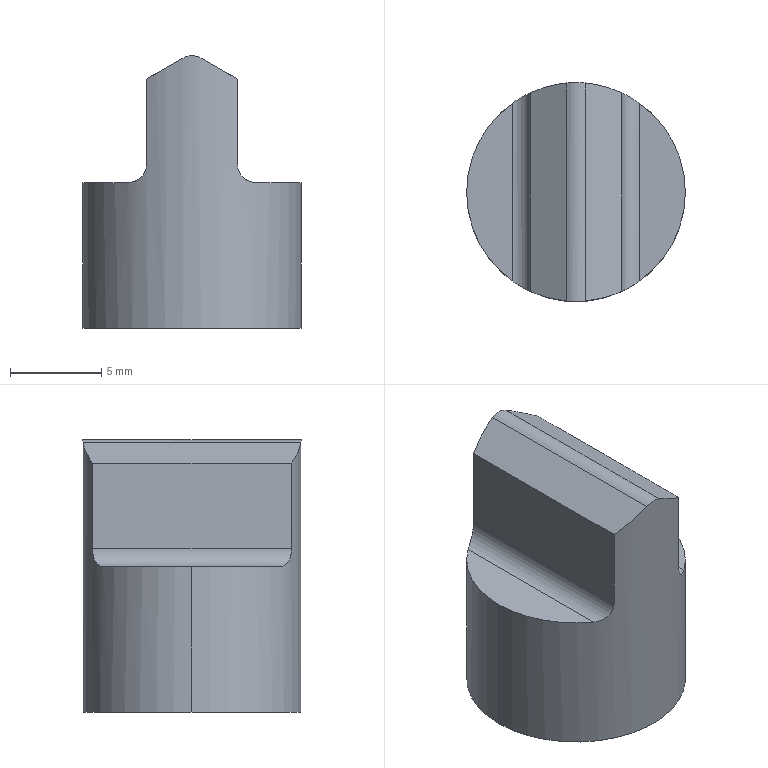Part | Creo | 1 solid | 15 faces | box 12 x 12 x 14.965 mm | volume 1022 mm3 | plane 8 | cylinder 7 | commonest cylinder face diameters 2 x3 10.5 x2 12 x2
STEP:
#1=CARTESIAN_POINT('',(257.5,-185.454,-31.823));
#2=VERTEX_POINT('',#1);
#3=CARTESIAN_POINT('',(257.5,-185.454,-36.5));
#4=VERTEX_POINT('',#3);
#5=CARTESIAN_POINT('',(257.5,-185.454,-31.823));
#6=DIRECTION('',(0.,0.,-1.));
#7=VECTOR('',#6,4.677);
#8=LINE('',#5,#7);
#9=EDGE_CURVE('',#2,#4,#8,.T.);
#10=ORIENTED_EDGE('',*,*,#9,.T.);
#11=CARTESIAN_POINT('',(257.5,-174.546,-36.5));
#12=VERTEX_POINT('',#11);
#13=CARTESIAN_POINT('',(257.5,-185.454,-36.5));
#14=DIRECTION('',(0.,1.,0.));
#15=VECTOR('',#14,10.909);
#16=LINE('',#13,#15);
#17=EDGE_CURVE('',#4,#12,#16,.T.);
#18=ORIENTED_EDGE('',*,*,#17,.T.);
#19=CARTESIAN_POINT('',(257.5,-174.546,-31.823));
#20=VERTEX_POINT('',#19);
#21=CARTESIAN_POINT('',(257.5,-174.546,-36.5));
#22=DIRECTION('',(0.,0.,1.));
#23=VECTOR('',#22,4.677);
#24=LINE('',#21,#23);
#25=EDGE_CURVE('',#12,#20,#24,.T.);
#26=ORIENTED_EDGE('',*,*,#25,.T.);
#27=CARTESIAN_POINT('',(257.5,-174.546,-31.823));
#28=DIRECTION('',(0.,-1.,0.));
#29=VECTOR('',#28,10.909);
#30=LINE('',#27,#29);
#31=EDGE_CURVE('',#20,#2,#30,.T.);
#32=ORIENTED_EDGE('',*,*,#31,.T.);
#33=EDGE_LOOP('',(#10,#18,#26,#32));
#34=FACE_OUTER_BOUND('',#33,.F.);
#35=CARTESIAN_POINT('',(257.5,-180.,-45.5));
#36=DIRECTION('',(1.,0.,0.));
#37=DIRECTION('',(0.,0.,-1.));
#38=AXIS2_PLACEMENT_3D('',#35,#36,#37);
#39=PLANE('',#38);
#40=ADVANCED_FACE('',(#34),#39,.F.);
#41=CARTESIAN_POINT('',(263.5,-184.873,-37.5));
#42=VERTEX_POINT('',#41);
#43=CARTESIAN_POINT('',(266.,-180.,-37.5));
#44=VERTEX_POINT('',#43);
#45=CARTESIAN_POINT('',(260.,-180.,-37.5));
#46=DIRECTION('',(0.,0.,1.));
#47=DIRECTION('',(0.5833,-0.8122,0.));
#48=AXIS2_PLACEMENT_3D('',#45,#46,#47);
#49=CIRCLE('',#48,6.);
#50=EDGE_CURVE('',#42,#44,#49,.T.);
#51=ORIENTED_EDGE('',*,*,#50,.T.);
#52=CARTESIAN_POINT('',(266.,-180.,-45.5));
#53=VERTEX_POINT('',#52);
#54=CARTESIAN_POINT('',(266.,-180.,-45.5));
#55=DIRECTION('',(0.,0.,1.));
#56=VECTOR('',#55,8.);
#57=LINE('',#54,#56);
#58=EDGE_CURVE('',#53,#44,#57,.T.);
#59=ORIENTED_EDGE('',*,*,#58,.F.);
#60=CARTESIAN_POINT('',(254.,-180.,-45.5));
#61=VERTEX_POINT('',#60);
#62=CARTESIAN_POINT('',(260.,-180.,-45.5));
#63=DIRECTION('',(0.,0.,-1.));
#64=DIRECTION('',(1.,0.,0.));
#65=AXIS2_PLACEMENT_3D('',#62,#63,#64);
#66=CIRCLE('',#65,6.);
#67=EDGE_CURVE('',#53,#61,#66,.T.);
#68=ORIENTED_EDGE('',*,*,#67,.T.);
#69=CARTESIAN_POINT('',(254.,-180.,-37.5));
#70=VERTEX_POINT('',#69);
#71=CARTESIAN_POINT('',(254.,-180.,-45.5));
#72=DIRECTION('',(0.000002775,0.,1.));
#73=VECTOR('',#72,8.);
#74=LINE('',#71,#73);
#75=EDGE_CURVE('',#61,#70,#74,.T.);
#76=ORIENTED_EDGE('',*,*,#75,.T.);
#77=CARTESIAN_POINT('',(256.5,-184.873,-37.5));
#78=VERTEX_POINT('',#77);
#79=CARTESIAN_POINT('',(260.,-180.,-37.5));
#80=DIRECTION('',(0.,0.,1.));
#81=DIRECTION('',(-1.,0.,0.));
#82=AXIS2_PLACEMENT_3D('',#79,#80,#81);
#83=CIRCLE('',#82,6.);
#84=EDGE_CURVE('',#70,#78,#83,.T.);
#85=ORIENTED_EDGE('',*,*,#84,.T.);
#86=CARTESIAN_POINT('',(257.5,-185.454,-36.5));
#87=CARTESIAN_POINT('',(257.5,-185.454,-36.573));
#88=CARTESIAN_POINT('',(257.484,-185.447,-36.716));
#89=CARTESIAN_POINT('',(257.414,-185.414,-36.926));
#90=CARTESIAN_POINT('',(257.299,-185.358,-37.115));
#91=CARTESIAN_POINT('',(257.144,-185.278,-37.276));
#92=CARTESIAN_POINT('',(256.954,-185.171,-37.401));
#93=CARTESIAN_POINT('',(256.737,-185.038,-37.481));
#94=CARTESIAN_POINT('',(256.581,-184.932,-37.5));
#95=CARTESIAN_POINT('',(256.5,-184.873,-37.5));
#96=B_SPLINE_CURVE_WITH_KNOTS('',3,(#86,#87,#88,#89,#90,#91,#92,#93,#94,#95),.UNSPECIFIED.,.F.,.F.,(4,1,1,1,1,1,1,4),(0.,0.1429,0.2857,0.4286,0.5714,0.7143,0.8571,1.),.UNSPECIFIED.);
#97=EDGE_CURVE('',#4,#78,#96,.T.);
#98=ORIENTED_EDGE('',*,*,#97,.F.);
#99=ORIENTED_EDGE('',*,*,#9,.F.);
#100=CARTESIAN_POINT('',(259.5,-185.979,-30.669));
#101=VERTEX_POINT('',#100);
#102=CARTESIAN_POINT('',(259.5,-185.979,-30.669));
#103=CARTESIAN_POINT('',(258.81,-185.921,-31.067));
#104=CARTESIAN_POINT('',(258.143,-185.749,-31.452));
#105=CARTESIAN_POINT('',(257.5,-185.454,-31.823));
#106=B_SPLINE_CURVE_WITH_KNOTS('',3,(#102,#103,#104,#105),.UNSPECIFIED.,.F.,.F.,(4,4),(0.,1.),.UNSPECIFIED.);
#107=EDGE_CURVE('',#101,#2,#106,.T.);
#108=ORIENTED_EDGE('',*,*,#107,.F.);
#109=CARTESIAN_POINT('',(260.5,-185.979,-30.669));
#110=VERTEX_POINT('',#109);
#111=CARTESIAN_POINT('',(260.5,-185.979,-30.669));
#112=CARTESIAN_POINT('',(260.439,-185.984,-30.633));
#113=CARTESIAN_POINT('',(260.311,-185.993,-30.577));
#114=CARTESIAN_POINT('',(260.105,-186.,-30.533));
#115=CARTESIAN_POINT('',(259.896,-186.,-30.533));
#116=CARTESIAN_POINT('',(259.689,-185.993,-30.577));
#117=CARTESIAN_POINT('',(259.562,-185.984,-30.633));
#118=CARTESIAN_POINT('',(259.5,-185.979,-30.669));
#119=B_SPLINE_CURVE_WITH_KNOTS('',3,(#111,#112,#113,#114,#115,#116,#117,#118),.UNSPECIFIED.,.F.,.F.,(4,1,1,1,1,4),(0.,0.2,0.4,0.6,0.8,1.),.UNSPECIFIED.);
#120=EDGE_CURVE('',#110,#101,#119,.T.);
#121=ORIENTED_EDGE('',*,*,#120,.F.);
#122=CARTESIAN_POINT('',(262.5,-185.454,-31.823));
#123=VERTEX_POINT('',#122);
#124=CARTESIAN_POINT('',(260.5,-185.979,-30.669));
#125=CARTESIAN_POINT('',(261.19,-185.921,-31.067));
#126=CARTESIAN_POINT('',(261.857,-185.749,-31.452));
#127=CARTESIAN_POINT('',(262.5,-185.454,-31.823));
#128=B_SPLINE_CURVE_WITH_KNOTS('',3,(#124,#125,#126,#127),.UNSPECIFIED.,.F.,.F.,(4,4),(0.,1.),.UNSPECIFIED.);
#129=EDGE_CURVE('',#110,#123,#128,.T.);
#130=ORIENTED_EDGE('',*,*,#129,.T.);
#131=CARTESIAN_POINT('',(262.5,-185.454,-36.5));
#132=VERTEX_POINT('',#131);
#133=CARTESIAN_POINT('',(262.5,-185.454,-36.5));
#134=DIRECTION('',(0.,0.,1.));
#135=VECTOR('',#134,4.677);
#136=LINE('',#133,#135);
#137=EDGE_CURVE('',#132,#123,#136,.T.);
#138=ORIENTED_EDGE('',*,*,#137,.F.);
#139=CARTESIAN_POINT('',(263.5,-184.873,-37.5));
#140=CARTESIAN_POINT('',(263.419,-184.932,-37.5));
#141=CARTESIAN_POINT('',(263.262,-185.038,-37.48));
#142=CARTESIAN_POINT('',(263.045,-185.172,-37.4));
#143=CARTESIAN_POINT('',(262.855,-185.278,-37.275));
#144=CARTESIAN_POINT('',(262.7,-185.359,-37.114));
#145=CARTESIAN_POINT('',(262.586,-185.414,-36.925));
#146=CARTESIAN_POINT('',(262.516,-185.447,-36.717));
#147=CARTESIAN_POINT('',(262.5,-185.454,-36.573));
#148=CARTESIAN_POINT('',(262.5,-185.454,-36.5));
#149=B_SPLINE_CURVE_WITH_KNOTS('',3,(#139,#140,#141,#142,#143,#144,#145,#146,#147,#148),.UNSPECIFIED.,.F.,.F.,(4,1,1,1,1,1,1,4),(0.,0.1429,0.2857,0.4286,0.5714,0.7143,0.8571,1.),.UNSPECIFIED.);
#150=EDGE_CURVE('',#42,#132,#149,.T.);
#151=ORIENTED_EDGE('',*,*,#150,.F.);
#152=EDGE_LOOP('',(#51,#59,#68,#76,#85,#98,#99,#108,#121,#130,#138,#151));
#153=FACE_OUTER_BOUND('',#152,.F.);
#154=CARTESIAN_POINT('',(260.,-180.,-53.5));
#155=DIRECTION('',(0.,0.,1.));
#156=DIRECTION('',(1.,0.,0.));
#157=AXIS2_PLACEMENT_3D('',#154,#155,#156);
#158=CYLINDRICAL_SURFACE('',#157,6.);
#159=ADVANCED_FACE('',(#153),#158,.T.);
#160=ORIENTED_EDGE('',*,*,#50,.F.);
#161=CARTESIAN_POINT('',(263.5,-175.127,-37.5));
#162=VERTEX_POINT('',#161);
#163=CARTESIAN_POINT('',(263.5,-184.873,-37.5));
#164=DIRECTION('',(0.,1.,0.));
#165=VECTOR('',#164,9.747);
#166=LINE('',#163,#165);
#167=EDGE_CURVE('',#42,#162,#166,.T.);
#168=ORIENTED_EDGE('',*,*,#167,.T.);
#169=CARTESIAN_POINT('',(260.,-180.,-37.5));
#170=DIRECTION('',(0.,0.,1.));
#171=DIRECTION('',(1.,0.,0.));
#172=AXIS2_PLACEMENT_3D('',#169,#170,#171);
#173=CIRCLE('',#172,6.);
#174=EDGE_CURVE('',#44,#162,#173,.T.);
#175=ORIENTED_EDGE('',*,*,#174,.F.);
#176=EDGE_LOOP('',(#160,#168,#175));
#177=FACE_OUTER_BOUND('',#176,.F.);
#178=CARTESIAN_POINT('',(260.,-180.,-37.5));
#179=DIRECTION('',(0.,0.,1.));
#180=DIRECTION('',(-1.,0.,0.));
#181=AXIS2_PLACEMENT_3D('',#178,#179,#180);
#182=PLANE('',#181);
#183=ADVANCED_FACE('',(#177),#182,.T.);
#184=CARTESIAN_POINT('',(262.5,-174.546,-36.5));
#185=VERTEX_POINT('',#184);
#186=CARTESIAN_POINT('',(262.5,-174.546,-36.5));
#187=CARTESIAN_POINT('',(262.5,-174.546,-36.573));
#188=CARTESIAN_POINT('',(262.516,-174.553,-36.716));
#189=CARTESIAN_POINT('',(262.586,-174.586,-36.926));
#190=CARTESIAN_POINT('',(262.701,-174.642,-37.115));
#191=CARTESIAN_POINT('',(262.856,-174.722,-37.276));
#192=CARTESIAN_POINT('',(263.046,-174.829,-37.401));
#193=CARTESIAN_POINT('',(263.263,-174.962,-37.481));
#194=CARTESIAN_POINT('',(263.419,-175.068,-37.5));
#195=CARTESIAN_POINT('',(263.5,-175.127,-37.5));
#196=B_SPLINE_CURVE_WITH_KNOTS('',3,(#186,#187,#188,#189,#190,#191,#192,#193,#194,#195),.UNSPECIFIED.,.F.,.F.,(4,1,1,1,1,1,1,4),(0.,0.1429,0.2857,0.4286,0.5714,0.7143,0.8571,1.),.UNSPECIFIED.);
#197=EDGE_CURVE('',#185,#162,#196,.T.);
#198=ORIENTED_EDGE('',*,*,#197,.T.);
#199=ORIENTED_EDGE('',*,*,#167,.F.);
#200=ORIENTED_EDGE('',*,*,#150,.T.);
#201=CARTESIAN_POINT('',(262.5,-174.546,-36.5));
#202=DIRECTION('',(0.,-1.,0.));
#203=VECTOR('',#202,10.909);
#204=LINE('',#201,#203);
#205=EDGE_CURVE('',#185,#132,#204,.T.);
#206=ORIENTED_EDGE('',*,*,#205,.F.);
#207=EDGE_LOOP('',(#198,#199,#200,#206));
#208=FACE_OUTER_BOUND('',#207,.F.);
#209=CARTESIAN_POINT('',(263.5,-180.,-36.5));
#210=DIRECTION('',(0.,-1.,0.));
#211=DIRECTION('',(0.,0.,-1.));
#212=AXIS2_PLACEMENT_3D('',#209,#210,#211);
#213=CYLINDRICAL_SURFACE('',#212,1.);
#214=ADVANCED_FACE('',(#208),#213,.F.);
#215=CARTESIAN_POINT('',(262.5,-174.546,-31.823));
#216=VERTEX_POINT('',#215);
#217=CARTESIAN_POINT('',(260.5,-174.021,-30.669));
#218=VERTEX_POINT('',#217);
#219=CARTESIAN_POINT('',(262.5,-174.546,-31.823));
#220=CARTESIAN_POINT('',(261.857,-174.251,-31.452));
#221=CARTESIAN_POINT('',(261.19,-174.079,-31.067));
#222=CARTESIAN_POINT('',(260.5,-174.021,-30.669));
#223=B_SPLINE_CURVE_WITH_KNOTS('',3,(#219,#220,#221,#222),.UNSPECIFIED.,.F.,.F.,(4,4),(0.,1.),.UNSPECIFIED.);
#224=EDGE_CURVE('',#216,#218,#223,.T.);
#225=ORIENTED_EDGE('',*,*,#224,.T.);
#226=CARTESIAN_POINT('',(259.5,-174.021,-30.669));
#227=VERTEX_POINT('',#226);
#228=CARTESIAN_POINT('',(259.5,-174.021,-30.669));
#229=CARTESIAN_POINT('',(259.561,-174.016,-30.633));
#230=CARTESIAN_POINT('',(259.689,-174.007,-30.577));
#231=CARTESIAN_POINT('',(259.895,-174.,-30.533));
#232=CARTESIAN_POINT('',(260.104,-174.,-30.533));
#233=CARTESIAN_POINT('',(260.311,-174.007,-30.577));
#234=CARTESIAN_POINT('',(260.438,-174.016,-30.633));
#235=CARTESIAN_POINT('',(260.5,-174.021,-30.669));
#236=B_SPLINE_CURVE_WITH_KNOTS('',3,(#228,#229,#230,#231,#232,#233,#234,#235),.UNSPECIFIED.,.F.,.F.,(4,1,1,1,1,4),(0.,0.2,0.4,0.6,0.8,1.),.UNSPECIFIED.);
#237=EDGE_CURVE('',#227,#218,#236,.T.);
#238=ORIENTED_EDGE('',*,*,#237,.F.);
#239=CARTESIAN_POINT('',(257.5,-174.546,-31.823));
#240=CARTESIAN_POINT('',(258.143,-174.251,-31.452));
#241=CARTESIAN_POINT('',(258.81,-174.079,-31.067));
#242=CARTESIAN_POINT('',(259.5,-174.021,-30.669));
#243=B_SPLINE_CURVE_WITH_KNOTS('',3,(#239,#240,#241,#242),.UNSPECIFIED.,.F.,.F.,(4,4),(0.,1.),.UNSPECIFIED.);
#244=EDGE_CURVE('',#20,#227,#243,.T.);
#245=ORIENTED_EDGE('',*,*,#244,.F.);
#246=ORIENTED_EDGE('',*,*,#25,.F.);
#247=CARTESIAN_POINT('',(256.5,-175.127,-37.5));
#248=VERTEX_POINT('',#247);
#249=CARTESIAN_POINT('',(256.5,-175.127,-37.5));
#250=CARTESIAN_POINT('',(256.581,-175.068,-37.5));
#251=CARTESIAN_POINT('',(256.738,-174.962,-37.48));
#252=CARTESIAN_POINT('',(256.955,-174.828,-37.4));
#253=CARTESIAN_POINT('',(257.145,-174.722,-37.275));
#254=CARTESIAN_POINT('',(257.3,-174.641,-37.114));
#255=CARTESIAN_POINT('',(257.414,-174.586,-36.925));
#256=CARTESIAN_POINT('',(257.484,-174.553,-36.717));
#257=CARTESIAN_POINT('',(257.5,-174.546,-36.573));
#258=CARTESIAN_POINT('',(257.5,-174.546,-36.5));
#259=B_SPLINE_CURVE_WITH_KNOTS('',3,(#249,#250,#251,#252,#253,#254,#255,#256,#257,#258),.UNSPECIFIED.,.F.,.F.,(4,1,1,1,1,1,1,4),(0.,0.1429,0.2857,0.4286,0.5714,0.7143,0.8571,1.),.UNSPECIFIED.);
#260=EDGE_CURVE('',#248,#12,#259,.T.);
#261=ORIENTED_EDGE('',*,*,#260,.F.);
#262=CARTESIAN_POINT('',(260.,-180.,-37.5));
#263=DIRECTION('',(0.,0.,1.));
#264=DIRECTION('',(-0.5833,0.8122,0.));
#265=AXIS2_PLACEMENT_3D('',#262,#263,#264);
#266=CIRCLE('',#265,6.);
#267=EDGE_CURVE('',#248,#70,#266,.T.);
#268=ORIENTED_EDGE('',*,*,#267,.T.);
#269=ORIENTED_EDGE('',*,*,#75,.F.);
#270=CARTESIAN_POINT('',(260.,-180.,-45.5));
#271=DIRECTION('',(0.,0.,-1.));
#272=DIRECTION('',(-1.,0.,0.));
#273=AXIS2_PLACEMENT_3D('',#270,#271,#272);
#274=CIRCLE('',#273,6.);
#275=EDGE_CURVE('',#61,#53,#274,.T.);
#276=ORIENTED_EDGE('',*,*,#275,.T.);
#277=ORIENTED_EDGE('',*,*,#58,.T.);
#278=ORIENTED_EDGE('',*,*,#174,.T.);
#279=ORIENTED_EDGE('',*,*,#197,.F.);
#280=CARTESIAN_POINT('',(262.5,-174.546,-31.823));
#281=DIRECTION('',(0.,0.,-1.));
#282=VECTOR('',#281,4.677);
#283=LINE('',#280,#282);
#284=EDGE_CURVE('',#216,#185,#283,.T.);
#285=ORIENTED_EDGE('',*,*,#284,.F.);
#286=EDGE_LOOP('',(#225,#238,#245,#246,#261,#268,#269,#276,#277,#278,#279,#285));
#287=FACE_OUTER_BOUND('',#286,.F.);
#288=CARTESIAN_POINT('',(260.,-180.,-53.5));
#289=DIRECTION('',(0.,0.,1.));
#290=DIRECTION('',(1.,0.,0.));
#291=AXIS2_PLACEMENT_3D('',#288,#289,#290);
#292=CYLINDRICAL_SURFACE('',#291,6.);
#293=ADVANCED_FACE('',(#287),#292,.T.);
#294=ORIENTED_EDGE('',*,*,#129,.F.);
#295=CARTESIAN_POINT('',(260.5,-185.979,-30.669));
#296=DIRECTION('',(0.,1.,0.));
#297=VECTOR('',#296,11.958);
#298=LINE('',#295,#297);
#299=EDGE_CURVE('',#110,#218,#298,.T.);
#300=ORIENTED_EDGE('',*,*,#299,.T.);
#301=ORIENTED_EDGE('',*,*,#224,.F.);
#302=CARTESIAN_POINT('',(262.5,-174.546,-31.823));
#303=DIRECTION('',(0.,-1.,0.));
#304=VECTOR('',#303,10.909);
#305=LINE('',#302,#304);
#306=EDGE_CURVE('',#216,#123,#305,.T.);
#307=ORIENTED_EDGE('',*,*,#306,.T.);
#308=EDGE_LOOP('',(#294,#300,#301,#307));
#309=FACE_OUTER_BOUND('',#308,.F.);
#310=CARTESIAN_POINT('',(260.,-180.,-30.38));
#311=DIRECTION('',(0.5,0.,0.866));
#312=DIRECTION('',(-0.866,0.,0.5));
#313=AXIS2_PLACEMENT_3D('',#310,#311,#312);
#314=PLANE('',#313);
#315=ADVANCED_FACE('',(#309),#314,.T.);
#316=ORIENTED_EDGE('',*,*,#120,.T.);
#317=CARTESIAN_POINT('',(259.5,-174.021,-30.669));
#318=DIRECTION('',(0.,-1.,0.));
#319=VECTOR('',#318,11.958);
#320=LINE('',#317,#319);
#321=EDGE_CURVE('',#227,#101,#320,.T.);
#322=ORIENTED_EDGE('',*,*,#321,.F.);
#323=ORIENTED_EDGE('',*,*,#237,.T.);
#324=ORIENTED_EDGE('',*,*,#299,.F.);
#325=EDGE_LOOP('',(#316,#322,#323,#324));
#326=FACE_OUTER_BOUND('',#325,.F.);
#327=CARTESIAN_POINT('',(260.,-180.,-31.535));
#328=DIRECTION('',(0.,1.,0.));
#329=DIRECTION('',(0.,0.,1.));
#330=AXIS2_PLACEMENT_3D('',#327,#328,#329);
#331=CYLINDRICAL_SURFACE('',#330,1.);
#332=ADVANCED_FACE('',(#326),#331,.T.);
#333=ORIENTED_EDGE('',*,*,#244,.T.);
#334=ORIENTED_EDGE('',*,*,#321,.T.);
#335=ORIENTED_EDGE('',*,*,#107,.T.);
#336=ORIENTED_EDGE('',*,*,#31,.F.);
#337=EDGE_LOOP('',(#333,#334,#335,#336));
#338=FACE_OUTER_BOUND('',#337,.F.);
#339=CARTESIAN_POINT('',(260.,-180.,-30.38));
#340=DIRECTION('',(-0.5,0.,0.866));
#341=DIRECTION('',(0.866,0.,0.5));
#342=AXIS2_PLACEMENT_3D('',#339,#340,#341);
#343=PLANE('',#342);
#344=ADVANCED_FACE('',(#338),#343,.T.);
#345=ORIENTED_EDGE('',*,*,#284,.T.);
#346=ORIENTED_EDGE('',*,*,#205,.T.);
#347=ORIENTED_EDGE('',*,*,#137,.T.);
#348=ORIENTED_EDGE('',*,*,#306,.F.);
#349=EDGE_LOOP('',(#345,#346,#347,#348));
#350=FACE_OUTER_BOUND('',#349,.F.);
#351=CARTESIAN_POINT('',(262.5,-180.,-45.5));
#352=DIRECTION('',(-1.,0.,0.));
#353=DIRECTION('',(0.,0.,-1.));
#354=AXIS2_PLACEMENT_3D('',#351,#352,#353);
#355=PLANE('',#354);
#356=ADVANCED_FACE('',(#350),#355,.F.);
#357=ORIENTED_EDGE('',*,*,#260,.T.);
#358=ORIENTED_EDGE('',*,*,#17,.F.);
#359=ORIENTED_EDGE('',*,*,#97,.T.);
#360=CARTESIAN_POINT('',(256.5,-175.127,-37.5));
#361=DIRECTION('',(0.,-1.,0.));
#362=VECTOR('',#361,9.747);
#363=LINE('',#360,#362);
#364=EDGE_CURVE('',#248,#78,#363,.T.);
#365=ORIENTED_EDGE('',*,*,#364,.F.);
#366=EDGE_LOOP('',(#357,#358,#359,#365));
#367=FACE_OUTER_BOUND('',#366,.F.);
#368=CARTESIAN_POINT('',(256.5,-180.,-36.5));
#369=DIRECTION('',(0.,-1.,0.));
#370=DIRECTION('',(0.,0.,-1.));
#371=AXIS2_PLACEMENT_3D('',#368,#369,#370);
#372=CYLINDRICAL_SURFACE('',#371,1.);
#373=ADVANCED_FACE('',(#367),#372,.F.);
#374=ORIENTED_EDGE('',*,*,#84,.F.);
#375=ORIENTED_EDGE('',*,*,#267,.F.);
#376=ORIENTED_EDGE('',*,*,#364,.T.);
#377=EDGE_LOOP('',(#374,#375,#376));
#378=FACE_OUTER_BOUND('',#377,.F.);
#379=CARTESIAN_POINT('',(260.,-180.,-37.5));
#380=DIRECTION('',(0.,0.,1.));
#381=DIRECTION('',(-1.,0.,0.));
#382=AXIS2_PLACEMENT_3D('',#379,#380,#381);
#383=PLANE('',#382);
#384=ADVANCED_FACE('',(#378),#383,.T.);
#385=ORIENTED_EDGE('',*,*,#275,.F.);
#386=ORIENTED_EDGE('',*,*,#67,.F.);
#387=EDGE_LOOP('',(#385,#386));
#388=FACE_OUTER_BOUND('',#387,.F.);
#389=CARTESIAN_POINT('',(254.75,-180.,-45.5));
#390=VERTEX_POINT('',#389);
#391=CARTESIAN_POINT('',(265.25,-180.,-45.5));
#392=VERTEX_POINT('',#391);
#393=CARTESIAN_POINT('',(260.,-180.,-45.5));
#394=DIRECTION('',(0.,0.,1.));
#395=DIRECTION('',(-1.,0.,0.));
#396=AXIS2_PLACEMENT_3D('',#393,#394,#395);
#397=CIRCLE('',#396,5.25);
#398=EDGE_CURVE('',#390,#392,#397,.T.);
#399=ORIENTED_EDGE('',*,*,#398,.F.);
#400=CARTESIAN_POINT('',(260.,-180.,-45.5));
#401=DIRECTION('',(0.,0.,1.));
#402=DIRECTION('',(1.,0.,0.));
#403=AXIS2_PLACEMENT_3D('',#400,#401,#402);
#404=CIRCLE('',#403,5.25);
#405=EDGE_CURVE('',#392,#390,#404,.T.);
#406=ORIENTED_EDGE('',*,*,#405,.F.);
#407=EDGE_LOOP('',(#399,#406));
#408=FACE_BOUND('',#407,.F.);
#409=CARTESIAN_POINT('',(260.,-180.,-45.5));
#410=DIRECTION('',(0.,0.,1.));
#411=DIRECTION('',(-1.,0.,0.));
#412=AXIS2_PLACEMENT_3D('',#409,#410,#411);
#413=PLANE('',#412);
#414=ADVANCED_FACE('',(#388,#408),#413,.F.);
#415=CARTESIAN_POINT('',(265.25,-180.,-42.5));
#416=VERTEX_POINT('',#415);
#417=CARTESIAN_POINT('',(254.75,-180.,-42.5));
#418=VERTEX_POINT('',#417);
#419=CARTESIAN_POINT('',(260.,-180.,-42.5));
#420=DIRECTION('',(0.,0.,-1.));
#421=DIRECTION('',(1.,0.,0.));
#422=AXIS2_PLACEMENT_3D('',#419,#420,#421);
#423=CIRCLE('',#422,5.25);
#424=EDGE_CURVE('',#416,#418,#423,.T.);
#425=ORIENTED_EDGE('',*,*,#424,.T.);
#426=CARTESIAN_POINT('',(254.75,-180.,-45.5));
#427=DIRECTION('',(0.,0.,1.));
#428=VECTOR('',#427,3.);
#429=LINE('',#426,#428);
#430=EDGE_CURVE('',#390,#418,#429,.T.);
#431=ORIENTED_EDGE('',*,*,#430,.F.);
#432=ORIENTED_EDGE('',*,*,#398,.T.);
#433=CARTESIAN_POINT('',(265.25,-180.,-45.5));
#434=DIRECTION('',(0.,0.,1.));
#435=VECTOR('',#434,3.);
#436=LINE('',#433,#435);
#437=EDGE_CURVE('',#392,#416,#436,.T.);
#438=ORIENTED_EDGE('',*,*,#437,.T.);
#439=EDGE_LOOP('',(#425,#431,#432,#438));
#440=FACE_OUTER_BOUND('',#439,.F.);
#441=CARTESIAN_POINT('',(260.,-180.,-45.5));
#442=DIRECTION('',(0.,0.,1.));
#443=DIRECTION('',(-1.,0.,0.));
#444=AXIS2_PLACEMENT_3D('',#441,#442,#443);
#445=CYLINDRICAL_SURFACE('',#444,5.25);
#446=ADVANCED_FACE('',(#440),#445,.F.);
#447=ORIENTED_EDGE('',*,*,#424,.F.);
#448=CARTESIAN_POINT('',(260.,-180.,-42.5));
#449=DIRECTION('',(0.,0.,-1.));
#450=DIRECTION('',(-1.,0.,0.));
#451=AXIS2_PLACEMENT_3D('',#448,#449,#450);
#452=CIRCLE('',#451,5.25);
#453=EDGE_CURVE('',#418,#416,#452,.T.);
#454=ORIENTED_EDGE('',*,*,#453,.F.);
#455=EDGE_LOOP('',(#447,#454));
#456=FACE_OUTER_BOUND('',#455,.F.);
#457=CARTESIAN_POINT('',(260.,-180.,-42.5));
#458=DIRECTION('',(0.,0.,1.));
#459=DIRECTION('',(-1.,0.,0.));
#460=AXIS2_PLACEMENT_3D('',#457,#458,#459);
#461=PLANE('',#460);
#462=ADVANCED_FACE('',(#456),#461,.F.);
#463=ORIENTED_EDGE('',*,*,#453,.T.);
#464=ORIENTED_EDGE('',*,*,#437,.F.);
#465=ORIENTED_EDGE('',*,*,#405,.T.);
#466=ORIENTED_EDGE('',*,*,#430,.T.);
#467=EDGE_LOOP('',(#463,#464,#465,#466));
#468=FACE_OUTER_BOUND('',#467,.F.);
#469=CARTESIAN_POINT('',(260.,-180.,-45.5));
#470=DIRECTION('',(0.,0.,1.));
#471=DIRECTION('',(-1.,0.,0.));
#472=AXIS2_PLACEMENT_3D('',#469,#470,#471);
#473=CYLINDRICAL_SURFACE('',#472,5.25);
#474=ADVANCED_FACE('',(#468),#473,.F.);
#475=CLOSED_SHELL('',(#40,#159,#183,#214,#293,#315,#332,#344,#356,#373,#384,#414,#446,#462,#474));
#476=MANIFOLD_SOLID_BREP('',#475);
#477=(LENGTH_UNIT()NAMED_UNIT(*)SI_UNIT(.MILLI.,.METRE.));
#478=UNCERTAINTY_MEASURE_WITH_UNIT(LENGTH_MEASURE(0.002263),#477,'','');
#479=(NAMED_UNIT(*)PLANE_ANGLE_UNIT()SI_UNIT($,.RADIAN.));
#480=PLANE_ANGLE_MEASURE_WITH_UNIT(PLANE_ANGLE_MEASURE(0.01745),#479);
#481=(CONVERSION_BASED_UNIT('DEGREE',#480)NAMED_UNIT(*)PLANE_ANGLE_UNIT());
#482=(NAMED_UNIT(*)SI_UNIT($,.STERADIAN.)SOLID_ANGLE_UNIT());
#483=(GEOMETRIC_REPRESENTATION_CONTEXT(3)GLOBAL_UNCERTAINTY_ASSIGNED_CONTEXT((#478))GLOBAL_UNIT_ASSIGNED_CONTEXT((#477,#481,#482))REPRESENTATION_CONTEXT('',''));
#484=ADVANCED_BREP_SHAPE_REPRESENTATION('',(#476),#483);